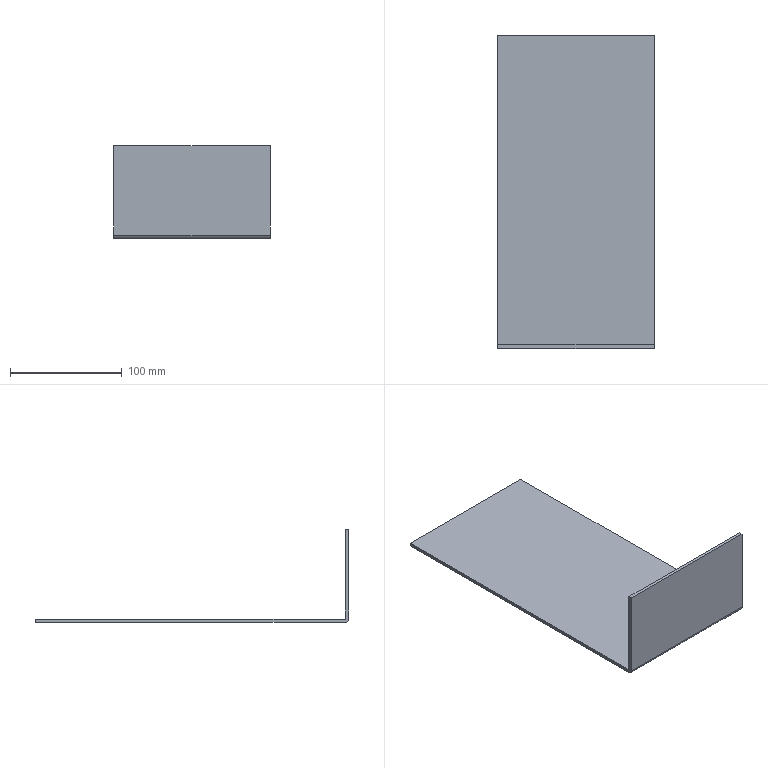Part | SolidWorks | features Extrusion 1, Fillet 1, ICE 1 | 1 solid | 9 faces | box 140 x 280 x 83 mm | volume 150930 mm3 | plane 8 | cylinder 1 | commonest cylinder face diameters 6 x1
STEP:
#1=CARTESIAN_POINT('',(140.,-277.,0.));
#2=VERTEX_POINT('',#1);
#3=CARTESIAN_POINT('',(0.,-277.,0.));
#4=VERTEX_POINT('',#3);
#5=CARTESIAN_POINT('',(0.,-277.,0.));
#6=DIRECTION('',(-1.,0.,0.));
#7=VECTOR('',#6,1000.);
#8=LINE('',#5,#7);
#9=EDGE_CURVE('',#2,#4,#8,.T.);
#10=ORIENTED_EDGE('',*,*,#9,.F.);
#11=CARTESIAN_POINT('',(140.,-280.,3.));
#12=VERTEX_POINT('',#11);
#13=CARTESIAN_POINT('',(140.,-277.,3.));
#14=DIRECTION('',(1.,0.,0.));
#15=DIRECTION('',(0.,-1.,0.));
#16=AXIS2_PLACEMENT_3D('',#13,#14,#15);
#17=CIRCLE('',#16,3.);
#18=EDGE_CURVE('',#12,#2,#17,.T.);
#19=ORIENTED_EDGE('',*,*,#18,.F.);
#20=CARTESIAN_POINT('',(0.,-280.,3.));
#21=VERTEX_POINT('',#20);
#22=CARTESIAN_POINT('',(0.,-280.,3.));
#23=DIRECTION('',(1.,0.,0.));
#24=VECTOR('',#23,1000.);
#25=LINE('',#22,#24);
#26=EDGE_CURVE('',#21,#12,#25,.T.);
#27=ORIENTED_EDGE('',*,*,#26,.F.);
#28=CARTESIAN_POINT('',(0.,-277.,3.));
#29=DIRECTION('',(-1.,0.,0.));
#30=DIRECTION('',(0.,0.,-1.));
#31=AXIS2_PLACEMENT_3D('',#28,#29,#30);
#32=CIRCLE('',#31,3.);
#33=EDGE_CURVE('',#4,#21,#32,.T.);
#34=ORIENTED_EDGE('',*,*,#33,.F.);
#35=EDGE_LOOP('',(#10,#19,#27,#34));
#36=FACE_OUTER_BOUND('',#35,.T.);
#37=CARTESIAN_POINT('',(0.,-277.,3.));
#38=DIRECTION('',(1.,0.,0.));
#39=DIRECTION('',(0.,0.,-1.));
#40=AXIS2_PLACEMENT_3D('',#37,#38,#39);
#41=CYLINDRICAL_SURFACE('',#40,3.);
#42=ADVANCED_FACE('',(#36),#41,.T.);
#43=CARTESIAN_POINT('',(140.,-277.,3.));
#44=VERTEX_POINT('',#43);
#45=CARTESIAN_POINT('',(0.,-277.,3.));
#46=VERTEX_POINT('',#45);
#47=CARTESIAN_POINT('',(140.,-277.,3.));
#48=DIRECTION('',(-1.,0.,0.));
#49=VECTOR('',#48,1000.);
#50=LINE('',#47,#49);
#51=EDGE_CURVE('',#44,#46,#50,.T.);
#52=ORIENTED_EDGE('',*,*,#51,.F.);
#53=CARTESIAN_POINT('',(140.,0.,3.));
#54=VERTEX_POINT('',#53);
#55=CARTESIAN_POINT('',(140.,0.,3.));
#56=DIRECTION('',(0.,1.,0.));
#57=VECTOR('',#56,1000.);
#58=LINE('',#55,#57);
#59=EDGE_CURVE('',#44,#54,#58,.T.);
#60=ORIENTED_EDGE('',*,*,#59,.T.);
#61=CARTESIAN_POINT('',(0.,0.,3.));
#62=VERTEX_POINT('',#61);
#63=CARTESIAN_POINT('',(0.,0.,3.));
#64=DIRECTION('',(-1.,0.,0.));
#65=VECTOR('',#64,1000.);
#66=LINE('',#63,#65);
#67=EDGE_CURVE('',#54,#62,#66,.T.);
#68=ORIENTED_EDGE('',*,*,#67,.T.);
#69=CARTESIAN_POINT('',(0.,-280.,3.));
#70=DIRECTION('',(0.,-1.,0.));
#71=VECTOR('',#70,1000.);
#72=LINE('',#69,#71);
#73=EDGE_CURVE('',#62,#46,#72,.T.);
#74=ORIENTED_EDGE('',*,*,#73,.T.);
#75=EDGE_LOOP('',(#52,#60,#68,#74));
#76=FACE_OUTER_BOUND('',#75,.T.);
#77=CARTESIAN_POINT('',(0.,0.,3.));
#78=DIRECTION('',(0.,0.,-1.));
#79=DIRECTION('',(-1.,0.,0.));
#80=AXIS2_PLACEMENT_3D('',#77,#78,#79);
#81=PLANE('',#80);
#82=ADVANCED_FACE('',(#76),#81,.F.);
#83=CARTESIAN_POINT('',(0.,0.,0.));
#84=VERTEX_POINT('',#83);
#85=CARTESIAN_POINT('',(0.,-280.,0.));
#86=DIRECTION('',(0.,-1.,0.));
#87=VECTOR('',#86,1000.);
#88=LINE('',#85,#87);
#89=EDGE_CURVE('',#84,#4,#88,.T.);
#90=ORIENTED_EDGE('',*,*,#89,.T.);
#91=ORIENTED_EDGE('',*,*,#33,.T.);
#92=CARTESIAN_POINT('',(0.,-280.,83.));
#93=VERTEX_POINT('',#92);
#94=CARTESIAN_POINT('',(0.,-280.,3.));
#95=DIRECTION('',(0.,0.,-1.));
#96=VECTOR('',#95,1000.);
#97=LINE('',#94,#96);
#98=EDGE_CURVE('',#93,#21,#97,.T.);
#99=ORIENTED_EDGE('',*,*,#98,.F.);
#100=CARTESIAN_POINT('',(0.,-277.,83.));
#101=VERTEX_POINT('',#100);
#102=CARTESIAN_POINT('',(0.,-277.,83.));
#103=DIRECTION('',(0.,-1.,0.));
#104=VECTOR('',#103,1000.);
#105=LINE('',#102,#104);
#106=EDGE_CURVE('',#101,#93,#105,.T.);
#107=ORIENTED_EDGE('',*,*,#106,.F.);
#108=CARTESIAN_POINT('',(0.,-277.,83.));
#109=DIRECTION('',(0.,0.,-1.));
#110=VECTOR('',#109,1000.);
#111=LINE('',#108,#110);
#112=EDGE_CURVE('',#101,#46,#111,.T.);
#113=ORIENTED_EDGE('',*,*,#112,.T.);
#114=ORIENTED_EDGE('',*,*,#73,.F.);
#115=CARTESIAN_POINT('',(0.,0.,3.));
#116=DIRECTION('',(0.,0.,-1.));
#117=VECTOR('',#116,1000.);
#118=LINE('',#115,#117);
#119=EDGE_CURVE('',#62,#84,#118,.T.);
#120=ORIENTED_EDGE('',*,*,#119,.T.);
#121=EDGE_LOOP('',(#90,#91,#99,#107,#113,#114,#120));
#122=FACE_OUTER_BOUND('',#121,.T.);
#123=CARTESIAN_POINT('',(0.,-280.,3.));
#124=DIRECTION('',(1.,0.,0.));
#125=DIRECTION('',(0.,0.,-1.));
#126=AXIS2_PLACEMENT_3D('',#123,#124,#125);
#127=PLANE('',#126);
#128=ADVANCED_FACE('',(#122),#127,.F.);
#129=ORIENTED_EDGE('',*,*,#98,.T.);
#130=ORIENTED_EDGE('',*,*,#26,.T.);
#131=CARTESIAN_POINT('',(140.,-280.,83.));
#132=VERTEX_POINT('',#131);
#133=CARTESIAN_POINT('',(140.,-280.,3.));
#134=DIRECTION('',(0.,0.,-1.));
#135=VECTOR('',#134,1000.);
#136=LINE('',#133,#135);
#137=EDGE_CURVE('',#132,#12,#136,.T.);
#138=ORIENTED_EDGE('',*,*,#137,.F.);
#139=CARTESIAN_POINT('',(0.,-280.,83.));
#140=DIRECTION('',(1.,0.,0.));
#141=VECTOR('',#140,1000.);
#142=LINE('',#139,#141);
#143=EDGE_CURVE('',#93,#132,#142,.T.);
#144=ORIENTED_EDGE('',*,*,#143,.F.);
#145=EDGE_LOOP('',(#129,#130,#138,#144));
#146=FACE_OUTER_BOUND('',#145,.T.);
#147=CARTESIAN_POINT('',(140.,-280.,3.));
#148=DIRECTION('',(0.,1.,0.));
#149=DIRECTION('',(0.,0.,1.));
#150=AXIS2_PLACEMENT_3D('',#147,#148,#149);
#151=PLANE('',#150);
#152=ADVANCED_FACE('',(#146),#151,.F.);
#153=ORIENTED_EDGE('',*,*,#137,.T.);
#154=ORIENTED_EDGE('',*,*,#18,.T.);
#155=CARTESIAN_POINT('',(140.,0.,0.));
#156=VERTEX_POINT('',#155);
#157=CARTESIAN_POINT('',(140.,0.,0.));
#158=DIRECTION('',(0.,1.,0.));
#159=VECTOR('',#158,1000.);
#160=LINE('',#157,#159);
#161=EDGE_CURVE('',#2,#156,#160,.T.);
#162=ORIENTED_EDGE('',*,*,#161,.T.);
#163=CARTESIAN_POINT('',(140.,0.,3.));
#164=DIRECTION('',(0.,0.,-1.));
#165=VECTOR('',#164,1000.);
#166=LINE('',#163,#165);
#167=EDGE_CURVE('',#54,#156,#166,.T.);
#168=ORIENTED_EDGE('',*,*,#167,.F.);
#169=ORIENTED_EDGE('',*,*,#59,.F.);
#170=CARTESIAN_POINT('',(140.,-277.,83.));
#171=VERTEX_POINT('',#170);
#172=CARTESIAN_POINT('',(140.,-277.,83.));
#173=DIRECTION('',(0.,0.,-1.));
#174=VECTOR('',#173,1000.);
#175=LINE('',#172,#174);
#176=EDGE_CURVE('',#171,#44,#175,.T.);
#177=ORIENTED_EDGE('',*,*,#176,.F.);
#178=CARTESIAN_POINT('',(140.,-280.,83.));
#179=DIRECTION('',(0.,1.,0.));
#180=VECTOR('',#179,1000.);
#181=LINE('',#178,#180);
#182=EDGE_CURVE('',#132,#171,#181,.T.);
#183=ORIENTED_EDGE('',*,*,#182,.F.);
#184=EDGE_LOOP('',(#153,#154,#162,#168,#169,#177,#183));
#185=FACE_OUTER_BOUND('',#184,.T.);
#186=CARTESIAN_POINT('',(140.,0.,3.));
#187=DIRECTION('',(-1.,0.,0.));
#188=DIRECTION('',(0.,-1.,0.));
#189=AXIS2_PLACEMENT_3D('',#186,#187,#188);
#190=PLANE('',#189);
#191=ADVANCED_FACE('',(#185),#190,.F.);
#192=CARTESIAN_POINT('',(0.,0.,0.));
#193=DIRECTION('',(-1.,0.,0.));
#194=VECTOR('',#193,1000.);
#195=LINE('',#192,#194);
#196=EDGE_CURVE('',#156,#84,#195,.T.);
#197=ORIENTED_EDGE('',*,*,#196,.T.);
#198=ORIENTED_EDGE('',*,*,#119,.F.);
#199=ORIENTED_EDGE('',*,*,#67,.F.);
#200=ORIENTED_EDGE('',*,*,#167,.T.);
#201=EDGE_LOOP('',(#197,#198,#199,#200));
#202=FACE_OUTER_BOUND('',#201,.T.);
#203=CARTESIAN_POINT('',(0.,0.,3.));
#204=DIRECTION('',(0.,-1.,0.));
#205=DIRECTION('',(0.,0.,-1.));
#206=AXIS2_PLACEMENT_3D('',#203,#204,#205);
#207=PLANE('',#206);
#208=ADVANCED_FACE('',(#202),#207,.F.);
#209=ORIENTED_EDGE('',*,*,#161,.F.);
#210=ORIENTED_EDGE('',*,*,#9,.T.);
#211=ORIENTED_EDGE('',*,*,#89,.F.);
#212=ORIENTED_EDGE('',*,*,#196,.F.);
#213=EDGE_LOOP('',(#209,#210,#211,#212));
#214=FACE_OUTER_BOUND('',#213,.T.);
#215=CARTESIAN_POINT('',(0.,0.,0.));
#216=DIRECTION('',(0.,0.,-1.));
#217=DIRECTION('',(-1.,0.,0.));
#218=AXIS2_PLACEMENT_3D('',#215,#216,#217);
#219=PLANE('',#218);
#220=ADVANCED_FACE('',(#214),#219,.T.);
#221=ORIENTED_EDGE('',*,*,#51,.T.);
#222=ORIENTED_EDGE('',*,*,#112,.F.);
#223=CARTESIAN_POINT('',(140.,-277.,83.));
#224=DIRECTION('',(-1.,0.,0.));
#225=VECTOR('',#224,1000.);
#226=LINE('',#223,#225);
#227=EDGE_CURVE('',#171,#101,#226,.T.);
#228=ORIENTED_EDGE('',*,*,#227,.F.);
#229=ORIENTED_EDGE('',*,*,#176,.T.);
#230=EDGE_LOOP('',(#221,#222,#228,#229));
#231=FACE_OUTER_BOUND('',#230,.T.);
#232=CARTESIAN_POINT('',(140.,-277.,83.));
#233=DIRECTION('',(0.,-1.,0.));
#234=DIRECTION('',(0.,0.,-1.));
#235=AXIS2_PLACEMENT_3D('',#232,#233,#234);
#236=PLANE('',#235);
#237=ADVANCED_FACE('',(#231),#236,.F.);
#238=ORIENTED_EDGE('',*,*,#143,.T.);
#239=ORIENTED_EDGE('',*,*,#182,.T.);
#240=ORIENTED_EDGE('',*,*,#227,.T.);
#241=ORIENTED_EDGE('',*,*,#106,.T.);
#242=EDGE_LOOP('',(#238,#239,#240,#241));
#243=FACE_OUTER_BOUND('',#242,.T.);
#244=CARTESIAN_POINT('',(0.,0.,83.));
#245=DIRECTION('',(0.,0.,1.));
#246=DIRECTION('',(1.,0.,0.));
#247=AXIS2_PLACEMENT_3D('',#244,#245,#246);
#248=PLANE('',#247);
#249=ADVANCED_FACE('',(#243),#248,.T.);
#250=CLOSED_SHELL('',(#42,#82,#128,#152,#191,#208,#220,#237,#249));
#251=MANIFOLD_SOLID_BREP('',#250);
#252=CARTESIAN_POINT('',(0.,0.,0.));
#253=DIRECTION('',(0.,0.,1.));
#254=DIRECTION('',(1.,0.,0.));
#255=AXIS2_PLACEMENT_3D('',#252,#253,#254);
#256=(LENGTH_UNIT()NAMED_UNIT(*)SI_UNIT(.MILLI.,.METRE.));
#257=UNCERTAINTY_MEASURE_WITH_UNIT(LENGTH_MEASURE(0.00001),#256,'','');
#258=(NAMED_UNIT(*)PLANE_ANGLE_UNIT()SI_UNIT($,.RADIAN.));
#259=(NAMED_UNIT(*)SI_UNIT($,.STERADIAN.)SOLID_ANGLE_UNIT());
#260=(GEOMETRIC_REPRESENTATION_CONTEXT(3)GLOBAL_UNCERTAINTY_ASSIGNED_CONTEXT((#257))GLOBAL_UNIT_ASSIGNED_CONTEXT((#256,#258,#259))REPRESENTATION_CONTEXT('',''));
#261=ADVANCED_BREP_SHAPE_REPRESENTATION('',(#251,#255),#260);